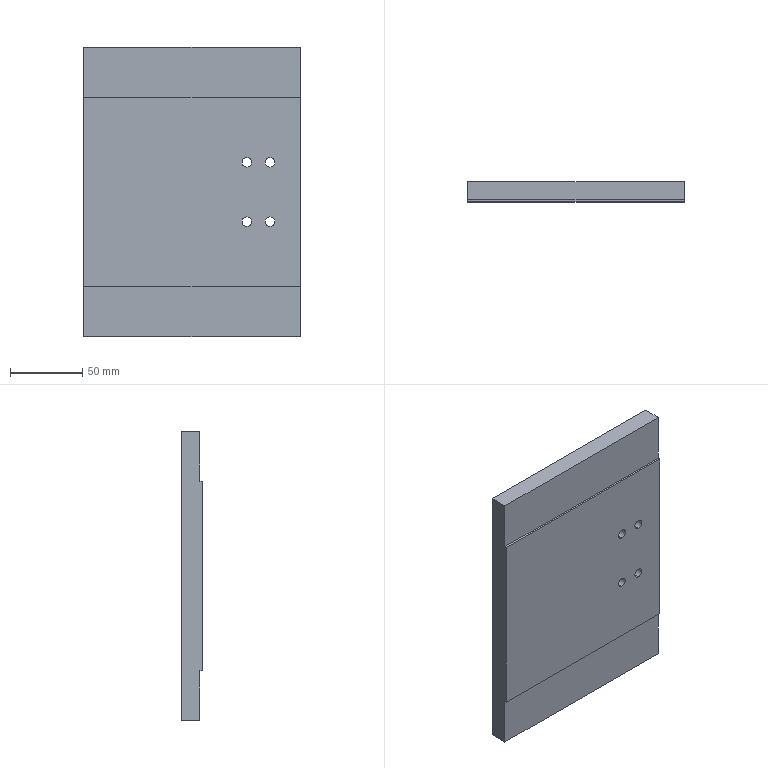Part | SolidWorks | features ICE 2, 3DProfileFeature 1, Extrusion 1, HoleWzd 1 | 1 solid | 30 faces | box 150 x 14 x 200 mm | volume 400905 mm3 | cylinder 16 | plane 14 | commonest cylinder face diameters 6.6 x8 11 x8
STEP:
#1=CARTESIAN_POINT('',(37.95,7.2,15.));
#2=VERTEX_POINT('',#1);
#3=CARTESIAN_POINT('',(37.95,7.2,26.));
#4=VERTEX_POINT('',#3);
#5=CARTESIAN_POINT('',(37.95,7.2,20.5));
#6=DIRECTION('',(0.,1.,0.));
#7=DIRECTION('',(0.,0.,1.));
#8=AXIS2_PLACEMENT_3D('',#5,#6,#7);
#9=CIRCLE('',#8,5.5);
#10=EDGE_CURVE('',#2,#4,#9,.T.);
#11=ORIENTED_EDGE('',*,*,#10,.F.);
#12=CARTESIAN_POINT('',(37.95,14.,15.));
#13=VERTEX_POINT('',#12);
#14=CARTESIAN_POINT('',(37.95,14.,15.));
#15=DIRECTION('',(0.,1.,0.));
#16=VECTOR('',#15,1000.);
#17=LINE('',#14,#16);
#18=EDGE_CURVE('',#2,#13,#17,.T.);
#19=ORIENTED_EDGE('',*,*,#18,.T.);
#20=CARTESIAN_POINT('',(37.95,14.,26.));
#21=VERTEX_POINT('',#20);
#22=CARTESIAN_POINT('',(37.95,14.,20.5));
#23=DIRECTION('',(0.,1.,0.));
#24=DIRECTION('',(0.,0.,1.));
#25=AXIS2_PLACEMENT_3D('',#22,#23,#24);
#26=CIRCLE('',#25,5.5);
#27=EDGE_CURVE('',#13,#21,#26,.T.);
#28=ORIENTED_EDGE('',*,*,#27,.T.);
#29=CARTESIAN_POINT('',(37.95,14.,26.));
#30=DIRECTION('',(0.,1.,0.));
#31=VECTOR('',#30,1000.);
#32=LINE('',#29,#31);
#33=EDGE_CURVE('',#4,#21,#32,.T.);
#34=ORIENTED_EDGE('',*,*,#33,.F.);
#35=EDGE_LOOP('',(#11,#19,#28,#34));
#36=FACE_OUTER_BOUND('',#35,.T.);
#37=CARTESIAN_POINT('',(37.95,14.,20.5));
#38=DIRECTION('',(0.,1.,0.));
#39=DIRECTION('',(0.,0.,1.));
#40=AXIS2_PLACEMENT_3D('',#37,#38,#39);
#41=CYLINDRICAL_SURFACE('',#40,5.5);
#42=ADVANCED_FACE('',(#36),#41,.F.);
#43=CARTESIAN_POINT('',(37.95,0.,23.8));
#44=VERTEX_POINT('',#43);
#45=CARTESIAN_POINT('',(37.95,0.,17.2));
#46=VERTEX_POINT('',#45);
#47=CARTESIAN_POINT('',(37.95,0.,20.5));
#48=DIRECTION('',(0.,-1.,0.));
#49=DIRECTION('',(0.,0.,-1.));
#50=AXIS2_PLACEMENT_3D('',#47,#48,#49);
#51=CIRCLE('',#50,3.3);
#52=EDGE_CURVE('',#44,#46,#51,.T.);
#53=ORIENTED_EDGE('',*,*,#52,.T.);
#54=CARTESIAN_POINT('',(37.95,7.2,17.2));
#55=VERTEX_POINT('',#54);
#56=CARTESIAN_POINT('',(37.95,14.,17.2));
#57=DIRECTION('',(0.,1.,0.));
#58=VECTOR('',#57,1000.);
#59=LINE('',#56,#58);
#60=EDGE_CURVE('',#46,#55,#59,.T.);
#61=ORIENTED_EDGE('',*,*,#60,.T.);
#62=CARTESIAN_POINT('',(37.95,7.2,23.8));
#63=VERTEX_POINT('',#62);
#64=CARTESIAN_POINT('',(37.95,7.2,20.5));
#65=DIRECTION('',(0.,1.,0.));
#66=DIRECTION('',(0.,0.,1.));
#67=AXIS2_PLACEMENT_3D('',#64,#65,#66);
#68=CIRCLE('',#67,3.3);
#69=EDGE_CURVE('',#55,#63,#68,.T.);
#70=ORIENTED_EDGE('',*,*,#69,.T.);
#71=CARTESIAN_POINT('',(37.95,14.,23.8));
#72=DIRECTION('',(0.,1.,0.));
#73=VECTOR('',#72,1000.);
#74=LINE('',#71,#73);
#75=EDGE_CURVE('',#44,#63,#74,.T.);
#76=ORIENTED_EDGE('',*,*,#75,.F.);
#77=EDGE_LOOP('',(#53,#61,#70,#76));
#78=FACE_OUTER_BOUND('',#77,.T.);
#79=CARTESIAN_POINT('',(37.95,14.,20.5));
#80=DIRECTION('',(0.,1.,0.));
#81=DIRECTION('',(0.,0.,1.));
#82=AXIS2_PLACEMENT_3D('',#79,#80,#81);
#83=CYLINDRICAL_SURFACE('',#82,3.3);
#84=ADVANCED_FACE('',(#78),#83,.F.);
#85=CARTESIAN_POINT('',(37.95,7.2,-26.));
#86=VERTEX_POINT('',#85);
#87=CARTESIAN_POINT('',(37.95,7.2,-15.));
#88=VERTEX_POINT('',#87);
#89=CARTESIAN_POINT('',(37.95,7.2,-20.5));
#90=DIRECTION('',(0.,1.,0.));
#91=DIRECTION('',(0.,0.,1.));
#92=AXIS2_PLACEMENT_3D('',#89,#90,#91);
#93=CIRCLE('',#92,5.5);
#94=EDGE_CURVE('',#86,#88,#93,.T.);
#95=ORIENTED_EDGE('',*,*,#94,.F.);
#96=CARTESIAN_POINT('',(37.95,14.,-26.));
#97=VERTEX_POINT('',#96);
#98=CARTESIAN_POINT('',(37.95,14.,-26.));
#99=DIRECTION('',(0.,1.,0.));
#100=VECTOR('',#99,1000.);
#101=LINE('',#98,#100);
#102=EDGE_CURVE('',#86,#97,#101,.T.);
#103=ORIENTED_EDGE('',*,*,#102,.T.);
#104=CARTESIAN_POINT('',(37.95,14.,-15.));
#105=VERTEX_POINT('',#104);
#106=CARTESIAN_POINT('',(37.95,14.,-20.5));
#107=DIRECTION('',(0.,1.,0.));
#108=DIRECTION('',(0.,0.,1.));
#109=AXIS2_PLACEMENT_3D('',#106,#107,#108);
#110=CIRCLE('',#109,5.5);
#111=EDGE_CURVE('',#97,#105,#110,.T.);
#112=ORIENTED_EDGE('',*,*,#111,.T.);
#113=CARTESIAN_POINT('',(37.95,14.,-15.));
#114=DIRECTION('',(0.,1.,0.));
#115=VECTOR('',#114,1000.);
#116=LINE('',#113,#115);
#117=EDGE_CURVE('',#88,#105,#116,.T.);
#118=ORIENTED_EDGE('',*,*,#117,.F.);
#119=EDGE_LOOP('',(#95,#103,#112,#118));
#120=FACE_OUTER_BOUND('',#119,.T.);
#121=CARTESIAN_POINT('',(37.95,14.,-20.5));
#122=DIRECTION('',(0.,1.,0.));
#123=DIRECTION('',(0.,0.,1.));
#124=AXIS2_PLACEMENT_3D('',#121,#122,#123);
#125=CYLINDRICAL_SURFACE('',#124,5.5);
#126=ADVANCED_FACE('',(#120),#125,.F.);
#127=CARTESIAN_POINT('',(37.95,0.,-17.2));
#128=VERTEX_POINT('',#127);
#129=CARTESIAN_POINT('',(37.95,0.,-23.8));
#130=VERTEX_POINT('',#129);
#131=CARTESIAN_POINT('',(37.95,0.,-20.5));
#132=DIRECTION('',(0.,-1.,0.));
#133=DIRECTION('',(0.,0.,-1.));
#134=AXIS2_PLACEMENT_3D('',#131,#132,#133);
#135=CIRCLE('',#134,3.3);
#136=EDGE_CURVE('',#128,#130,#135,.T.);
#137=ORIENTED_EDGE('',*,*,#136,.T.);
#138=CARTESIAN_POINT('',(37.95,7.2,-23.8));
#139=VERTEX_POINT('',#138);
#140=CARTESIAN_POINT('',(37.95,14.,-23.8));
#141=DIRECTION('',(0.,1.,0.));
#142=VECTOR('',#141,1000.);
#143=LINE('',#140,#142);
#144=EDGE_CURVE('',#130,#139,#143,.T.);
#145=ORIENTED_EDGE('',*,*,#144,.T.);
#146=CARTESIAN_POINT('',(37.95,7.2,-17.2));
#147=VERTEX_POINT('',#146);
#148=CARTESIAN_POINT('',(37.95,7.2,-20.5));
#149=DIRECTION('',(0.,1.,0.));
#150=DIRECTION('',(0.,0.,1.));
#151=AXIS2_PLACEMENT_3D('',#148,#149,#150);
#152=CIRCLE('',#151,3.3);
#153=EDGE_CURVE('',#139,#147,#152,.T.);
#154=ORIENTED_EDGE('',*,*,#153,.T.);
#155=CARTESIAN_POINT('',(37.95,14.,-17.2));
#156=DIRECTION('',(0.,1.,0.));
#157=VECTOR('',#156,1000.);
#158=LINE('',#155,#157);
#159=EDGE_CURVE('',#128,#147,#158,.T.);
#160=ORIENTED_EDGE('',*,*,#159,.F.);
#161=EDGE_LOOP('',(#137,#145,#154,#160));
#162=FACE_OUTER_BOUND('',#161,.T.);
#163=CARTESIAN_POINT('',(37.95,14.,-20.5));
#164=DIRECTION('',(0.,1.,0.));
#165=DIRECTION('',(0.,0.,1.));
#166=AXIS2_PLACEMENT_3D('',#163,#164,#165);
#167=CYLINDRICAL_SURFACE('',#166,3.3);
#168=ADVANCED_FACE('',(#162),#167,.F.);
#169=CARTESIAN_POINT('',(53.95,7.2,15.));
#170=VERTEX_POINT('',#169);
#171=CARTESIAN_POINT('',(53.95,7.2,26.));
#172=VERTEX_POINT('',#171);
#173=CARTESIAN_POINT('',(53.95,7.2,20.5));
#174=DIRECTION('',(0.,1.,0.));
#175=DIRECTION('',(0.,0.,1.));
#176=AXIS2_PLACEMENT_3D('',#173,#174,#175);
#177=CIRCLE('',#176,5.5);
#178=EDGE_CURVE('',#170,#172,#177,.T.);
#179=ORIENTED_EDGE('',*,*,#178,.F.);
#180=CARTESIAN_POINT('',(53.95,14.,15.));
#181=VERTEX_POINT('',#180);
#182=CARTESIAN_POINT('',(53.95,14.,15.));
#183=DIRECTION('',(0.,1.,0.));
#184=VECTOR('',#183,1000.);
#185=LINE('',#182,#184);
#186=EDGE_CURVE('',#170,#181,#185,.T.);
#187=ORIENTED_EDGE('',*,*,#186,.T.);
#188=CARTESIAN_POINT('',(53.95,14.,26.));
#189=VERTEX_POINT('',#188);
#190=CARTESIAN_POINT('',(53.95,14.,20.5));
#191=DIRECTION('',(0.,1.,0.));
#192=DIRECTION('',(0.,0.,1.));
#193=AXIS2_PLACEMENT_3D('',#190,#191,#192);
#194=CIRCLE('',#193,5.5);
#195=EDGE_CURVE('',#181,#189,#194,.T.);
#196=ORIENTED_EDGE('',*,*,#195,.T.);
#197=CARTESIAN_POINT('',(53.95,14.,26.));
#198=DIRECTION('',(0.,1.,0.));
#199=VECTOR('',#198,1000.);
#200=LINE('',#197,#199);
#201=EDGE_CURVE('',#172,#189,#200,.T.);
#202=ORIENTED_EDGE('',*,*,#201,.F.);
#203=EDGE_LOOP('',(#179,#187,#196,#202));
#204=FACE_OUTER_BOUND('',#203,.T.);
#205=CARTESIAN_POINT('',(53.95,14.,20.5));
#206=DIRECTION('',(0.,1.,0.));
#207=DIRECTION('',(0.,0.,1.));
#208=AXIS2_PLACEMENT_3D('',#205,#206,#207);
#209=CYLINDRICAL_SURFACE('',#208,5.5);
#210=ADVANCED_FACE('',(#204),#209,.F.);
#211=CARTESIAN_POINT('',(53.95,0.,23.8));
#212=VERTEX_POINT('',#211);
#213=CARTESIAN_POINT('',(53.95,0.,17.2));
#214=VERTEX_POINT('',#213);
#215=CARTESIAN_POINT('',(53.95,0.,20.5));
#216=DIRECTION('',(0.,-1.,0.));
#217=DIRECTION('',(0.,0.,-1.));
#218=AXIS2_PLACEMENT_3D('',#215,#216,#217);
#219=CIRCLE('',#218,3.3);
#220=EDGE_CURVE('',#212,#214,#219,.T.);
#221=ORIENTED_EDGE('',*,*,#220,.T.);
#222=CARTESIAN_POINT('',(53.95,7.2,17.2));
#223=VERTEX_POINT('',#222);
#224=CARTESIAN_POINT('',(53.95,14.,17.2));
#225=DIRECTION('',(0.,1.,0.));
#226=VECTOR('',#225,1000.);
#227=LINE('',#224,#226);
#228=EDGE_CURVE('',#214,#223,#227,.T.);
#229=ORIENTED_EDGE('',*,*,#228,.T.);
#230=CARTESIAN_POINT('',(53.95,7.2,23.8));
#231=VERTEX_POINT('',#230);
#232=CARTESIAN_POINT('',(53.95,7.2,20.5));
#233=DIRECTION('',(0.,1.,0.));
#234=DIRECTION('',(0.,0.,1.));
#235=AXIS2_PLACEMENT_3D('',#232,#233,#234);
#236=CIRCLE('',#235,3.3);
#237=EDGE_CURVE('',#223,#231,#236,.T.);
#238=ORIENTED_EDGE('',*,*,#237,.T.);
#239=CARTESIAN_POINT('',(53.95,14.,23.8));
#240=DIRECTION('',(0.,1.,0.));
#241=VECTOR('',#240,1000.);
#242=LINE('',#239,#241);
#243=EDGE_CURVE('',#212,#231,#242,.T.);
#244=ORIENTED_EDGE('',*,*,#243,.F.);
#245=EDGE_LOOP('',(#221,#229,#238,#244));
#246=FACE_OUTER_BOUND('',#245,.T.);
#247=CARTESIAN_POINT('',(53.95,14.,20.5));
#248=DIRECTION('',(0.,1.,0.));
#249=DIRECTION('',(0.,0.,1.));
#250=AXIS2_PLACEMENT_3D('',#247,#248,#249);
#251=CYLINDRICAL_SURFACE('',#250,3.3);
#252=ADVANCED_FACE('',(#246),#251,.F.);
#253=CARTESIAN_POINT('',(53.95,7.2,-26.));
#254=VERTEX_POINT('',#253);
#255=CARTESIAN_POINT('',(53.95,7.2,-15.));
#256=VERTEX_POINT('',#255);
#257=CARTESIAN_POINT('',(53.95,7.2,-20.5));
#258=DIRECTION('',(0.,1.,0.));
#259=DIRECTION('',(0.,0.,1.));
#260=AXIS2_PLACEMENT_3D('',#257,#258,#259);
#261=CIRCLE('',#260,5.5);
#262=EDGE_CURVE('',#254,#256,#261,.T.);
#263=ORIENTED_EDGE('',*,*,#262,.F.);
#264=CARTESIAN_POINT('',(53.95,14.,-26.));
#265=VERTEX_POINT('',#264);
#266=CARTESIAN_POINT('',(53.95,14.,-26.));
#267=DIRECTION('',(0.,1.,0.));
#268=VECTOR('',#267,1000.);
#269=LINE('',#266,#268);
#270=EDGE_CURVE('',#254,#265,#269,.T.);
#271=ORIENTED_EDGE('',*,*,#270,.T.);
#272=CARTESIAN_POINT('',(53.95,14.,-15.));
#273=VERTEX_POINT('',#272);
#274=CARTESIAN_POINT('',(53.95,14.,-20.5));
#275=DIRECTION('',(0.,1.,0.));
#276=DIRECTION('',(0.,0.,1.));
#277=AXIS2_PLACEMENT_3D('',#274,#275,#276);
#278=CIRCLE('',#277,5.5);
#279=EDGE_CURVE('',#265,#273,#278,.T.);
#280=ORIENTED_EDGE('',*,*,#279,.T.);
#281=CARTESIAN_POINT('',(53.95,14.,-15.));
#282=DIRECTION('',(0.,1.,0.));
#283=VECTOR('',#282,1000.);
#284=LINE('',#281,#283);
#285=EDGE_CURVE('',#256,#273,#284,.T.);
#286=ORIENTED_EDGE('',*,*,#285,.F.);
#287=EDGE_LOOP('',(#263,#271,#280,#286));
#288=FACE_OUTER_BOUND('',#287,.T.);
#289=CARTESIAN_POINT('',(53.95,14.,-20.5));
#290=DIRECTION('',(0.,1.,0.));
#291=DIRECTION('',(0.,0.,1.));
#292=AXIS2_PLACEMENT_3D('',#289,#290,#291);
#293=CYLINDRICAL_SURFACE('',#292,5.5);
#294=ADVANCED_FACE('',(#288),#293,.F.);
#295=CARTESIAN_POINT('',(53.95,0.,-17.2));
#296=VERTEX_POINT('',#295);
#297=CARTESIAN_POINT('',(53.95,0.,-23.8));
#298=VERTEX_POINT('',#297);
#299=CARTESIAN_POINT('',(53.95,0.,-20.5));
#300=DIRECTION('',(0.,-1.,0.));
#301=DIRECTION('',(0.,0.,-1.));
#302=AXIS2_PLACEMENT_3D('',#299,#300,#301);
#303=CIRCLE('',#302,3.3);
#304=EDGE_CURVE('',#296,#298,#303,.T.);
#305=ORIENTED_EDGE('',*,*,#304,.T.);
#306=CARTESIAN_POINT('',(53.95,7.2,-23.8));
#307=VERTEX_POINT('',#306);
#308=CARTESIAN_POINT('',(53.95,14.,-23.8));
#309=DIRECTION('',(0.,1.,0.));
#310=VECTOR('',#309,1000.);
#311=LINE('',#308,#310);
#312=EDGE_CURVE('',#298,#307,#311,.T.);
#313=ORIENTED_EDGE('',*,*,#312,.T.);
#314=CARTESIAN_POINT('',(53.95,7.2,-17.2));
#315=VERTEX_POINT('',#314);
#316=CARTESIAN_POINT('',(53.95,7.2,-20.5));
#317=DIRECTION('',(0.,1.,0.));
#318=DIRECTION('',(0.,0.,1.));
#319=AXIS2_PLACEMENT_3D('',#316,#317,#318);
#320=CIRCLE('',#319,3.3);
#321=EDGE_CURVE('',#307,#315,#320,.T.);
#322=ORIENTED_EDGE('',*,*,#321,.T.);
#323=CARTESIAN_POINT('',(53.95,14.,-17.2));
#324=DIRECTION('',(0.,1.,0.));
#325=VECTOR('',#324,1000.);
#326=LINE('',#323,#325);
#327=EDGE_CURVE('',#296,#315,#326,.T.);
#328=ORIENTED_EDGE('',*,*,#327,.F.);
#329=EDGE_LOOP('',(#305,#313,#322,#328));
#330=FACE_OUTER_BOUND('',#329,.T.);
#331=CARTESIAN_POINT('',(53.95,14.,-20.5));
#332=DIRECTION('',(0.,1.,0.));
#333=DIRECTION('',(0.,0.,1.));
#334=AXIS2_PLACEMENT_3D('',#331,#332,#333);
#335=CYLINDRICAL_SURFACE('',#334,3.3);
#336=ADVANCED_FACE('',(#330),#335,.F.);
#337=CARTESIAN_POINT('',(75.,1.5,100.));
#338=VERTEX_POINT('',#337);
#339=CARTESIAN_POINT('',(-75.,1.5,100.));
#340=VERTEX_POINT('',#339);
#341=CARTESIAN_POINT('',(-75.,1.5,100.));
#342=DIRECTION('',(-1.,0.,0.));
#343=VECTOR('',#342,1000.);
#344=LINE('',#341,#343);
#345=EDGE_CURVE('',#338,#340,#344,.T.);
#346=ORIENTED_EDGE('',*,*,#345,.F.);
#347=CARTESIAN_POINT('',(75.,14.,100.));
#348=VERTEX_POINT('',#347);
#349=CARTESIAN_POINT('',(75.,14.,100.));
#350=DIRECTION('',(0.,-1.,0.));
#351=VECTOR('',#350,1000.);
#352=LINE('',#349,#351);
#353=EDGE_CURVE('',#348,#338,#352,.T.);
#354=ORIENTED_EDGE('',*,*,#353,.F.);
#355=CARTESIAN_POINT('',(-75.,14.,100.));
#356=VERTEX_POINT('',#355);
#357=CARTESIAN_POINT('',(-75.,14.,100.));
#358=DIRECTION('',(1.,0.,0.));
#359=VECTOR('',#358,1000.);
#360=LINE('',#357,#359);
#361=EDGE_CURVE('',#356,#348,#360,.T.);
#362=ORIENTED_EDGE('',*,*,#361,.F.);
#363=CARTESIAN_POINT('',(-75.,14.,100.));
#364=DIRECTION('',(0.,-1.,0.));
#365=VECTOR('',#364,1000.);
#366=LINE('',#363,#365);
#367=EDGE_CURVE('',#356,#340,#366,.T.);
#368=ORIENTED_EDGE('',*,*,#367,.T.);
#369=EDGE_LOOP('',(#346,#354,#362,#368));
#370=FACE_OUTER_BOUND('',#369,.T.);
#371=CARTESIAN_POINT('',(-75.,14.,100.));
#372=DIRECTION('',(0.,0.,-1.));
#373=DIRECTION('',(-1.,0.,0.));
#374=AXIS2_PLACEMENT_3D('',#371,#372,#373);
#375=PLANE('',#374);
#376=ADVANCED_FACE('',(#370),#375,.F.);
#377=CARTESIAN_POINT('',(75.,1.5,65.5));
#378=VERTEX_POINT('',#377);
#379=CARTESIAN_POINT('',(75.,1.5,100.));
#380=DIRECTION('',(0.,0.,1.));
#381=VECTOR('',#380,1000.);
#382=LINE('',#379,#381);
#383=EDGE_CURVE('',#378,#338,#382,.T.);
#384=ORIENTED_EDGE('',*,*,#383,.F.);
#385=CARTESIAN_POINT('',(75.,0.,65.5));
#386=VERTEX_POINT('',#385);
#387=CARTESIAN_POINT('',(75.,1.5,65.5));
#388=DIRECTION('',(0.,-1.,0.));
#389=VECTOR('',#388,1000.);
#390=LINE('',#387,#389);
#391=EDGE_CURVE('',#378,#386,#390,.T.);
#392=ORIENTED_EDGE('',*,*,#391,.T.);
#393=CARTESIAN_POINT('',(75.,0.,-65.5));
#394=VERTEX_POINT('',#393);
#395=CARTESIAN_POINT('',(75.,0.,100.));
#396=DIRECTION('',(0.,0.,-1.));
#397=VECTOR('',#396,1000.);
#398=LINE('',#395,#397);
#399=EDGE_CURVE('',#386,#394,#398,.T.);
#400=ORIENTED_EDGE('',*,*,#399,.T.);
#401=CARTESIAN_POINT('',(75.,1.5,-65.5));
#402=VERTEX_POINT('',#401);
#403=CARTESIAN_POINT('',(75.,1.5,-65.5));
#404=DIRECTION('',(0.,-1.,0.));
#405=VECTOR('',#404,1000.);
#406=LINE('',#403,#405);
#407=EDGE_CURVE('',#402,#394,#406,.T.);
#408=ORIENTED_EDGE('',*,*,#407,.F.);
#409=CARTESIAN_POINT('',(75.,1.5,-100.));
#410=VERTEX_POINT('',#409);
#411=CARTESIAN_POINT('',(75.,1.5,-100.));
#412=DIRECTION('',(0.,0.,1.));
#413=VECTOR('',#412,1000.);
#414=LINE('',#411,#413);
#415=EDGE_CURVE('',#410,#402,#414,.T.);
#416=ORIENTED_EDGE('',*,*,#415,.F.);
#417=CARTESIAN_POINT('',(75.,14.,-100.));
#418=VERTEX_POINT('',#417);
#419=CARTESIAN_POINT('',(75.,14.,-100.));
#420=DIRECTION('',(0.,-1.,0.));
#421=VECTOR('',#420,1000.);
#422=LINE('',#419,#421);
#423=EDGE_CURVE('',#418,#410,#422,.T.);
#424=ORIENTED_EDGE('',*,*,#423,.F.);
#425=CARTESIAN_POINT('',(75.,14.,100.));
#426=DIRECTION('',(0.,0.,-1.));
#427=VECTOR('',#426,1000.);
#428=LINE('',#425,#427);
#429=EDGE_CURVE('',#348,#418,#428,.T.);
#430=ORIENTED_EDGE('',*,*,#429,.F.);
#431=ORIENTED_EDGE('',*,*,#353,.T.);
#432=EDGE_LOOP('',(#384,#392,#400,#408,#416,#424,#430,#431));
#433=FACE_OUTER_BOUND('',#432,.T.);
#434=CARTESIAN_POINT('',(75.,14.,100.));
#435=DIRECTION('',(-1.,0.,0.));
#436=DIRECTION('',(0.,0.,1.));
#437=AXIS2_PLACEMENT_3D('',#434,#435,#436);
#438=PLANE('',#437);
#439=ADVANCED_FACE('',(#433),#438,.F.);
#440=ORIENTED_EDGE('',*,*,#423,.T.);
#441=CARTESIAN_POINT('',(-75.,1.5,-100.));
#442=VERTEX_POINT('',#441);
#443=CARTESIAN_POINT('',(-75.,1.5,-100.));
#444=DIRECTION('',(1.,0.,0.));
#445=VECTOR('',#444,1000.);
#446=LINE('',#443,#445);
#447=EDGE_CURVE('',#442,#410,#446,.T.);
#448=ORIENTED_EDGE('',*,*,#447,.F.);
#449=CARTESIAN_POINT('',(-75.,14.,-100.));
#450=VERTEX_POINT('',#449);
#451=CARTESIAN_POINT('',(-75.,14.,-100.));
#452=DIRECTION('',(0.,-1.,0.));
#453=VECTOR('',#452,1000.);
#454=LINE('',#451,#453);
#455=EDGE_CURVE('',#450,#442,#454,.T.);
#456=ORIENTED_EDGE('',*,*,#455,.F.);
#457=CARTESIAN_POINT('',(-75.,14.,-100.));
#458=DIRECTION('',(-1.,0.,0.));
#459=VECTOR('',#458,1000.);
#460=LINE('',#457,#459);
#461=EDGE_CURVE('',#418,#450,#460,.T.);
#462=ORIENTED_EDGE('',*,*,#461,.F.);
#463=EDGE_LOOP('',(#440,#448,#456,#462));
#464=FACE_OUTER_BOUND('',#463,.T.);
#465=CARTESIAN_POINT('',(-75.,14.,-100.));
#466=DIRECTION('',(0.,0.,1.));
#467=DIRECTION('',(1.,0.,0.));
#468=AXIS2_PLACEMENT_3D('',#465,#466,#467);
#469=PLANE('',#468);
#470=ADVANCED_FACE('',(#464),#469,.F.);
#471=CARTESIAN_POINT('',(-75.,0.,-65.5));
#472=VERTEX_POINT('',#471);
#473=CARTESIAN_POINT('',(-75.,0.,65.5));
#474=VERTEX_POINT('',#473);
#475=CARTESIAN_POINT('',(-75.,0.,100.));
#476=DIRECTION('',(0.,0.,1.));
#477=VECTOR('',#476,1000.);
#478=LINE('',#475,#477);
#479=EDGE_CURVE('',#472,#474,#478,.T.);
#480=ORIENTED_EDGE('',*,*,#479,.T.);
#481=CARTESIAN_POINT('',(-75.,1.5,65.5));
#482=VERTEX_POINT('',#481);
#483=CARTESIAN_POINT('',(-75.,1.5,65.5));
#484=DIRECTION('',(0.,-1.,0.));
#485=VECTOR('',#484,1000.);
#486=LINE('',#483,#485);
#487=EDGE_CURVE('',#482,#474,#486,.T.);
#488=ORIENTED_EDGE('',*,*,#487,.F.);
#489=CARTESIAN_POINT('',(-75.,1.5,100.));
#490=DIRECTION('',(0.,0.,-1.));
#491=VECTOR('',#490,1000.);
#492=LINE('',#489,#491);
#493=EDGE_CURVE('',#340,#482,#492,.T.);
#494=ORIENTED_EDGE('',*,*,#493,.F.);
#495=ORIENTED_EDGE('',*,*,#367,.F.);
#496=CARTESIAN_POINT('',(-75.,14.,100.));
#497=DIRECTION('',(0.,0.,1.));
#498=VECTOR('',#497,1000.);
#499=LINE('',#496,#498);
#500=EDGE_CURVE('',#450,#356,#499,.T.);
#501=ORIENTED_EDGE('',*,*,#500,.F.);
#502=ORIENTED_EDGE('',*,*,#455,.T.);
#503=CARTESIAN_POINT('',(-75.,1.5,-65.5));
#504=VERTEX_POINT('',#503);
#505=CARTESIAN_POINT('',(-75.,1.5,-100.));
#506=DIRECTION('',(0.,0.,-1.));
#507=VECTOR('',#506,1000.);
#508=LINE('',#505,#507);
#509=EDGE_CURVE('',#504,#442,#508,.T.);
#510=ORIENTED_EDGE('',*,*,#509,.F.);
#511=CARTESIAN_POINT('',(-75.,1.5,-65.5));
#512=DIRECTION('',(0.,-1.,0.));
#513=VECTOR('',#512,1000.);
#514=LINE('',#511,#513);
#515=EDGE_CURVE('',#504,#472,#514,.T.);
#516=ORIENTED_EDGE('',*,*,#515,.T.);
#517=EDGE_LOOP('',(#480,#488,#494,#495,#501,#502,#510,#516));
#518=FACE_OUTER_BOUND('',#517,.T.);
#519=CARTESIAN_POINT('',(-75.,14.,100.));
#520=DIRECTION('',(1.,0.,0.));
#521=DIRECTION('',(0.,0.,-1.));
#522=AXIS2_PLACEMENT_3D('',#519,#520,#521);
#523=PLANE('',#522);
#524=ADVANCED_FACE('',(#518),#523,.F.);
#525=CARTESIAN_POINT('',(37.95,14.,20.5));
#526=DIRECTION('',(0.,1.,0.));
#527=DIRECTION('',(0.,0.,1.));
#528=AXIS2_PLACEMENT_3D('',#525,#526,#527);
#529=CIRCLE('',#528,5.5);
#530=EDGE_CURVE('',#21,#13,#529,.T.);
#531=ORIENTED_EDGE('',*,*,#530,.F.);
#532=ORIENTED_EDGE('',*,*,#27,.F.);
#533=EDGE_LOOP('',(#531,#532));
#534=FACE_BOUND('',#533,.T.);
#535=CARTESIAN_POINT('',(37.95,14.,-20.5));
#536=DIRECTION('',(0.,1.,0.));
#537=DIRECTION('',(0.,0.,1.));
#538=AXIS2_PLACEMENT_3D('',#535,#536,#537);
#539=CIRCLE('',#538,5.5);
#540=EDGE_CURVE('',#105,#97,#539,.T.);
#541=ORIENTED_EDGE('',*,*,#540,.F.);
#542=ORIENTED_EDGE('',*,*,#111,.F.);
#543=EDGE_LOOP('',(#541,#542));
#544=FACE_BOUND('',#543,.T.);
#545=CARTESIAN_POINT('',(53.95,14.,20.5));
#546=DIRECTION('',(0.,1.,0.));
#547=DIRECTION('',(0.,0.,1.));
#548=AXIS2_PLACEMENT_3D('',#545,#546,#547);
#549=CIRCLE('',#548,5.5);
#550=EDGE_CURVE('',#189,#181,#549,.T.);
#551=ORIENTED_EDGE('',*,*,#550,.F.);
#552=ORIENTED_EDGE('',*,*,#195,.F.);
#553=EDGE_LOOP('',(#551,#552));
#554=FACE_BOUND('',#553,.T.);
#555=CARTESIAN_POINT('',(53.95,14.,-20.5));
#556=DIRECTION('',(0.,1.,0.));
#557=DIRECTION('',(0.,0.,1.));
#558=AXIS2_PLACEMENT_3D('',#555,#556,#557);
#559=CIRCLE('',#558,5.5);
#560=EDGE_CURVE('',#273,#265,#559,.T.);
#561=ORIENTED_EDGE('',*,*,#560,.F.);
#562=ORIENTED_EDGE('',*,*,#279,.F.);
#563=EDGE_LOOP('',(#561,#562));
#564=FACE_BOUND('',#563,.T.);
#565=ORIENTED_EDGE('',*,*,#429,.T.);
#566=ORIENTED_EDGE('',*,*,#461,.T.);
#567=ORIENTED_EDGE('',*,*,#500,.T.);
#568=ORIENTED_EDGE('',*,*,#361,.T.);
#569=EDGE_LOOP('',(#565,#566,#567,#568));
#570=FACE_OUTER_BOUND('',#569,.T.);
#571=CARTESIAN_POINT('',(0.,14.,0.));
#572=DIRECTION('',(0.,-1.,0.));
#573=DIRECTION('',(0.,0.,-1.));
#574=AXIS2_PLACEMENT_3D('',#571,#572,#573);
#575=PLANE('',#574);
#576=ADVANCED_FACE('',(#534,#544,#554,#564,#570),#575,.F.);
#577=ORIENTED_EDGE('',*,*,#52,.F.);
#578=CARTESIAN_POINT('',(37.95,0.,20.5));
#579=DIRECTION('',(0.,-1.,0.));
#580=DIRECTION('',(0.,0.,-1.));
#581=AXIS2_PLACEMENT_3D('',#578,#579,#580);
#582=CIRCLE('',#581,3.3);
#583=EDGE_CURVE('',#46,#44,#582,.T.);
#584=ORIENTED_EDGE('',*,*,#583,.F.);
#585=EDGE_LOOP('',(#577,#584));
#586=FACE_BOUND('',#585,.T.);
#587=ORIENTED_EDGE('',*,*,#136,.F.);
#588=CARTESIAN_POINT('',(37.95,0.,-20.5));
#589=DIRECTION('',(0.,-1.,0.));
#590=DIRECTION('',(0.,0.,-1.));
#591=AXIS2_PLACEMENT_3D('',#588,#589,#590);
#592=CIRCLE('',#591,3.3);
#593=EDGE_CURVE('',#130,#128,#592,.T.);
#594=ORIENTED_EDGE('',*,*,#593,.F.);
#595=EDGE_LOOP('',(#587,#594));
#596=FACE_BOUND('',#595,.T.);
#597=ORIENTED_EDGE('',*,*,#220,.F.);
#598=CARTESIAN_POINT('',(53.95,0.,20.5));
#599=DIRECTION('',(0.,-1.,0.));
#600=DIRECTION('',(0.,0.,-1.));
#601=AXIS2_PLACEMENT_3D('',#598,#599,#600);
#602=CIRCLE('',#601,3.3);
#603=EDGE_CURVE('',#214,#212,#602,.T.);
#604=ORIENTED_EDGE('',*,*,#603,.F.);
#605=EDGE_LOOP('',(#597,#604));
#606=FACE_BOUND('',#605,.T.);
#607=ORIENTED_EDGE('',*,*,#304,.F.);
#608=CARTESIAN_POINT('',(53.95,0.,-20.5));
#609=DIRECTION('',(0.,-1.,0.));
#610=DIRECTION('',(0.,0.,-1.));
#611=AXIS2_PLACEMENT_3D('',#608,#609,#610);
#612=CIRCLE('',#611,3.3);
#613=EDGE_CURVE('',#298,#296,#612,.T.);
#614=ORIENTED_EDGE('',*,*,#613,.F.);
#615=EDGE_LOOP('',(#607,#614));
#616=FACE_BOUND('',#615,.T.);
#617=CARTESIAN_POINT('',(-75.,0.,65.5));
#618=DIRECTION('',(1.,0.,0.));
#619=VECTOR('',#618,1000.);
#620=LINE('',#617,#619);
#621=EDGE_CURVE('',#474,#386,#620,.T.);
#622=ORIENTED_EDGE('',*,*,#621,.F.);
#623=ORIENTED_EDGE('',*,*,#479,.F.);
#624=CARTESIAN_POINT('',(-75.,0.,-65.5));
#625=DIRECTION('',(-1.,0.,0.));
#626=VECTOR('',#625,1000.);
#627=LINE('',#624,#626);
#628=EDGE_CURVE('',#394,#472,#627,.T.);
#629=ORIENTED_EDGE('',*,*,#628,.F.);
#630=ORIENTED_EDGE('',*,*,#399,.F.);
#631=EDGE_LOOP('',(#622,#623,#629,#630));
#632=FACE_OUTER_BOUND('',#631,.T.);
#633=CARTESIAN_POINT('',(0.,0.,0.));
#634=DIRECTION('',(0.,-1.,0.));
#635=DIRECTION('',(0.,0.,-1.));
#636=AXIS2_PLACEMENT_3D('',#633,#634,#635);
#637=PLANE('',#636);
#638=ADVANCED_FACE('',(#586,#596,#606,#616,#632),#637,.T.);
#639=ORIENTED_EDGE('',*,*,#628,.T.);
#640=ORIENTED_EDGE('',*,*,#515,.F.);
#641=CARTESIAN_POINT('',(-75.,1.5,-65.5));
#642=DIRECTION('',(-1.,0.,0.));
#643=VECTOR('',#642,1000.);
#644=LINE('',#641,#643);
#645=EDGE_CURVE('',#402,#504,#644,.T.);
#646=ORIENTED_EDGE('',*,*,#645,.F.);
#647=ORIENTED_EDGE('',*,*,#407,.T.);
#648=EDGE_LOOP('',(#639,#640,#646,#647));
#649=FACE_OUTER_BOUND('',#648,.T.);
#650=CARTESIAN_POINT('',(-75.,1.5,-65.5));
#651=DIRECTION('',(0.,0.,1.));
#652=DIRECTION('',(1.,0.,0.));
#653=AXIS2_PLACEMENT_3D('',#650,#651,#652);
#654=PLANE('',#653);
#655=ADVANCED_FACE('',(#649),#654,.F.);
#656=ORIENTED_EDGE('',*,*,#509,.T.);
#657=ORIENTED_EDGE('',*,*,#447,.T.);
#658=ORIENTED_EDGE('',*,*,#415,.T.);
#659=ORIENTED_EDGE('',*,*,#645,.T.);
#660=EDGE_LOOP('',(#656,#657,#658,#659));
#661=FACE_OUTER_BOUND('',#660,.T.);
#662=CARTESIAN_POINT('',(0.,1.5,0.));
#663=DIRECTION('',(0.,1.,0.));
#664=DIRECTION('',(0.,0.,1.));
#665=AXIS2_PLACEMENT_3D('',#662,#663,#664);
#666=PLANE('',#665);
#667=ADVANCED_FACE('',(#661),#666,.F.);
#668=ORIENTED_EDGE('',*,*,#621,.T.);
#669=ORIENTED_EDGE('',*,*,#391,.F.);
#670=CARTESIAN_POINT('',(-75.,1.5,65.5));
#671=DIRECTION('',(1.,0.,0.));
#672=VECTOR('',#671,1000.);
#673=LINE('',#670,#672);
#674=EDGE_CURVE('',#482,#378,#673,.T.);
#675=ORIENTED_EDGE('',*,*,#674,.F.);
#676=ORIENTED_EDGE('',*,*,#487,.T.);
#677=EDGE_LOOP('',(#668,#669,#675,#676));
#678=FACE_OUTER_BOUND('',#677,.T.);
#679=CARTESIAN_POINT('',(-75.,1.5,65.5));
#680=DIRECTION('',(0.,0.,-1.));
#681=DIRECTION('',(-1.,0.,0.));
#682=AXIS2_PLACEMENT_3D('',#679,#680,#681);
#683=PLANE('',#682);
#684=ADVANCED_FACE('',(#678),#683,.F.);
#685=ORIENTED_EDGE('',*,*,#493,.T.);
#686=ORIENTED_EDGE('',*,*,#674,.T.);
#687=ORIENTED_EDGE('',*,*,#383,.T.);
#688=ORIENTED_EDGE('',*,*,#345,.T.);
#689=EDGE_LOOP('',(#685,#686,#687,#688));
#690=FACE_OUTER_BOUND('',#689,.T.);
#691=CARTESIAN_POINT('',(0.,1.5,0.));
#692=DIRECTION('',(0.,-1.,0.));
#693=DIRECTION('',(0.,0.,-1.));
#694=AXIS2_PLACEMENT_3D('',#691,#692,#693);
#695=PLANE('',#694);
#696=ADVANCED_FACE('',(#690),#695,.T.);
#697=ORIENTED_EDGE('',*,*,#312,.F.);
#698=ORIENTED_EDGE('',*,*,#613,.T.);
#699=ORIENTED_EDGE('',*,*,#327,.T.);
#700=CARTESIAN_POINT('',(53.95,7.2,-20.5));
#701=DIRECTION('',(0.,1.,0.));
#702=DIRECTION('',(0.,0.,1.));
#703=AXIS2_PLACEMENT_3D('',#700,#701,#702);
#704=CIRCLE('',#703,3.3);
#705=EDGE_CURVE('',#315,#307,#704,.T.);
#706=ORIENTED_EDGE('',*,*,#705,.T.);
#707=EDGE_LOOP('',(#697,#698,#699,#706));
#708=FACE_OUTER_BOUND('',#707,.T.);
#709=CARTESIAN_POINT('',(53.95,14.,-20.5));
#710=DIRECTION('',(0.,1.,0.));
#711=DIRECTION('',(0.,0.,1.));
#712=AXIS2_PLACEMENT_3D('',#709,#710,#711);
#713=CYLINDRICAL_SURFACE('',#712,3.3);
#714=ADVANCED_FACE('',(#708),#713,.F.);
#715=ORIENTED_EDGE('',*,*,#705,.F.);
#716=ORIENTED_EDGE('',*,*,#321,.F.);
#717=EDGE_LOOP('',(#715,#716));
#718=FACE_BOUND('',#717,.T.);
#719=CARTESIAN_POINT('',(53.95,7.2,-20.5));
#720=DIRECTION('',(0.,1.,0.));
#721=DIRECTION('',(0.,0.,1.));
#722=AXIS2_PLACEMENT_3D('',#719,#720,#721);
#723=CIRCLE('',#722,5.5);
#724=EDGE_CURVE('',#256,#254,#723,.T.);
#725=ORIENTED_EDGE('',*,*,#724,.T.);
#726=ORIENTED_EDGE('',*,*,#262,.T.);
#727=EDGE_LOOP('',(#725,#726));
#728=FACE_OUTER_BOUND('',#727,.T.);
#729=CARTESIAN_POINT('',(57.25,7.2,-20.5));
#730=DIRECTION('',(0.,-1.,0.));
#731=DIRECTION('',(0.,0.,-1.));
#732=AXIS2_PLACEMENT_3D('',#729,#730,#731);
#733=PLANE('',#732);
#734=ADVANCED_FACE('',(#718,#728),#733,.F.);
#735=ORIENTED_EDGE('',*,*,#270,.F.);
#736=ORIENTED_EDGE('',*,*,#724,.F.);
#737=ORIENTED_EDGE('',*,*,#285,.T.);
#738=ORIENTED_EDGE('',*,*,#560,.T.);
#739=EDGE_LOOP('',(#735,#736,#737,#738));
#740=FACE_OUTER_BOUND('',#739,.T.);
#741=CARTESIAN_POINT('',(53.95,14.,-20.5));
#742=DIRECTION('',(0.,1.,0.));
#743=DIRECTION('',(0.,0.,1.));
#744=AXIS2_PLACEMENT_3D('',#741,#742,#743);
#745=CYLINDRICAL_SURFACE('',#744,5.5);
#746=ADVANCED_FACE('',(#740),#745,.F.);
#747=ORIENTED_EDGE('',*,*,#228,.F.);
#748=ORIENTED_EDGE('',*,*,#603,.T.);
#749=ORIENTED_EDGE('',*,*,#243,.T.);
#750=CARTESIAN_POINT('',(53.95,7.2,20.5));
#751=DIRECTION('',(0.,1.,0.));
#752=DIRECTION('',(0.,0.,1.));
#753=AXIS2_PLACEMENT_3D('',#750,#751,#752);
#754=CIRCLE('',#753,3.3);
#755=EDGE_CURVE('',#231,#223,#754,.T.);
#756=ORIENTED_EDGE('',*,*,#755,.T.);
#757=EDGE_LOOP('',(#747,#748,#749,#756));
#758=FACE_OUTER_BOUND('',#757,.T.);
#759=CARTESIAN_POINT('',(53.95,14.,20.5));
#760=DIRECTION('',(0.,1.,0.));
#761=DIRECTION('',(0.,0.,1.));
#762=AXIS2_PLACEMENT_3D('',#759,#760,#761);
#763=CYLINDRICAL_SURFACE('',#762,3.3);
#764=ADVANCED_FACE('',(#758),#763,.F.);
#765=ORIENTED_EDGE('',*,*,#755,.F.);
#766=ORIENTED_EDGE('',*,*,#237,.F.);
#767=EDGE_LOOP('',(#765,#766));
#768=FACE_BOUND('',#767,.T.);
#769=CARTESIAN_POINT('',(53.95,7.2,20.5));
#770=DIRECTION('',(0.,1.,0.));
#771=DIRECTION('',(0.,0.,1.));
#772=AXIS2_PLACEMENT_3D('',#769,#770,#771);
#773=CIRCLE('',#772,5.5);
#774=EDGE_CURVE('',#172,#170,#773,.T.);
#775=ORIENTED_EDGE('',*,*,#774,.T.);
#776=ORIENTED_EDGE('',*,*,#178,.T.);
#777=EDGE_LOOP('',(#775,#776));
#778=FACE_OUTER_BOUND('',#777,.T.);
#779=CARTESIAN_POINT('',(57.25,7.2,20.5));
#780=DIRECTION('',(0.,-1.,0.));
#781=DIRECTION('',(0.,0.,-1.));
#782=AXIS2_PLACEMENT_3D('',#779,#780,#781);
#783=PLANE('',#782);
#784=ADVANCED_FACE('',(#768,#778),#783,.F.);
#785=ORIENTED_EDGE('',*,*,#186,.F.);
#786=ORIENTED_EDGE('',*,*,#774,.F.);
#787=ORIENTED_EDGE('',*,*,#201,.T.);
#788=ORIENTED_EDGE('',*,*,#550,.T.);
#789=EDGE_LOOP('',(#785,#786,#787,#788));
#790=FACE_OUTER_BOUND('',#789,.T.);
#791=CARTESIAN_POINT('',(53.95,14.,20.5));
#792=DIRECTION('',(0.,1.,0.));
#793=DIRECTION('',(0.,0.,1.));
#794=AXIS2_PLACEMENT_3D('',#791,#792,#793);
#795=CYLINDRICAL_SURFACE('',#794,5.5);
#796=ADVANCED_FACE('',(#790),#795,.F.);
#797=ORIENTED_EDGE('',*,*,#144,.F.);
#798=ORIENTED_EDGE('',*,*,#593,.T.);
#799=ORIENTED_EDGE('',*,*,#159,.T.);
#800=CARTESIAN_POINT('',(37.95,7.2,-20.5));
#801=DIRECTION('',(0.,1.,0.));
#802=DIRECTION('',(0.,0.,1.));
#803=AXIS2_PLACEMENT_3D('',#800,#801,#802);
#804=CIRCLE('',#803,3.3);
#805=EDGE_CURVE('',#147,#139,#804,.T.);
#806=ORIENTED_EDGE('',*,*,#805,.T.);
#807=EDGE_LOOP('',(#797,#798,#799,#806));
#808=FACE_OUTER_BOUND('',#807,.T.);
#809=CARTESIAN_POINT('',(37.95,14.,-20.5));
#810=DIRECTION('',(0.,1.,0.));
#811=DIRECTION('',(0.,0.,1.));
#812=AXIS2_PLACEMENT_3D('',#809,#810,#811);
#813=CYLINDRICAL_SURFACE('',#812,3.3);
#814=ADVANCED_FACE('',(#808),#813,.F.);
#815=ORIENTED_EDGE('',*,*,#805,.F.);
#816=ORIENTED_EDGE('',*,*,#153,.F.);
#817=EDGE_LOOP('',(#815,#816));
#818=FACE_BOUND('',#817,.T.);
#819=CARTESIAN_POINT('',(37.95,7.2,-20.5));
#820=DIRECTION('',(0.,1.,0.));
#821=DIRECTION('',(0.,0.,1.));
#822=AXIS2_PLACEMENT_3D('',#819,#820,#821);
#823=CIRCLE('',#822,5.5);
#824=EDGE_CURVE('',#88,#86,#823,.T.);
#825=ORIENTED_EDGE('',*,*,#824,.T.);
#826=ORIENTED_EDGE('',*,*,#94,.T.);
#827=EDGE_LOOP('',(#825,#826));
#828=FACE_OUTER_BOUND('',#827,.T.);
#829=CARTESIAN_POINT('',(41.25,7.2,-20.5));
#830=DIRECTION('',(0.,-1.,0.));
#831=DIRECTION('',(0.,0.,-1.));
#832=AXIS2_PLACEMENT_3D('',#829,#830,#831);
#833=PLANE('',#832);
#834=ADVANCED_FACE('',(#818,#828),#833,.F.);
#835=ORIENTED_EDGE('',*,*,#102,.F.);
#836=ORIENTED_EDGE('',*,*,#824,.F.);
#837=ORIENTED_EDGE('',*,*,#117,.T.);
#838=ORIENTED_EDGE('',*,*,#540,.T.);
#839=EDGE_LOOP('',(#835,#836,#837,#838));
#840=FACE_OUTER_BOUND('',#839,.T.);
#841=CARTESIAN_POINT('',(37.95,14.,-20.5));
#842=DIRECTION('',(0.,1.,0.));
#843=DIRECTION('',(0.,0.,1.));
#844=AXIS2_PLACEMENT_3D('',#841,#842,#843);
#845=CYLINDRICAL_SURFACE('',#844,5.5);
#846=ADVANCED_FACE('',(#840),#845,.F.);
#847=ORIENTED_EDGE('',*,*,#60,.F.);
#848=ORIENTED_EDGE('',*,*,#583,.T.);
#849=ORIENTED_EDGE('',*,*,#75,.T.);
#850=CARTESIAN_POINT('',(37.95,7.2,20.5));
#851=DIRECTION('',(0.,1.,0.));
#852=DIRECTION('',(0.,0.,1.));
#853=AXIS2_PLACEMENT_3D('',#850,#851,#852);
#854=CIRCLE('',#853,3.3);
#855=EDGE_CURVE('',#63,#55,#854,.T.);
#856=ORIENTED_EDGE('',*,*,#855,.T.);
#857=EDGE_LOOP('',(#847,#848,#849,#856));
#858=FACE_OUTER_BOUND('',#857,.T.);
#859=CARTESIAN_POINT('',(37.95,14.,20.5));
#860=DIRECTION('',(0.,1.,0.));
#861=DIRECTION('',(0.,0.,1.));
#862=AXIS2_PLACEMENT_3D('',#859,#860,#861);
#863=CYLINDRICAL_SURFACE('',#862,3.3);
#864=ADVANCED_FACE('',(#858),#863,.F.);
#865=ORIENTED_EDGE('',*,*,#855,.F.);
#866=ORIENTED_EDGE('',*,*,#69,.F.);
#867=EDGE_LOOP('',(#865,#866));
#868=FACE_BOUND('',#867,.T.);
#869=CARTESIAN_POINT('',(37.95,7.2,20.5));
#870=DIRECTION('',(0.,1.,0.));
#871=DIRECTION('',(0.,0.,1.));
#872=AXIS2_PLACEMENT_3D('',#869,#870,#871);
#873=CIRCLE('',#872,5.5);
#874=EDGE_CURVE('',#4,#2,#873,.T.);
#875=ORIENTED_EDGE('',*,*,#874,.T.);
#876=ORIENTED_EDGE('',*,*,#10,.T.);
#877=EDGE_LOOP('',(#875,#876));
#878=FACE_OUTER_BOUND('',#877,.T.);
#879=CARTESIAN_POINT('',(41.25,7.2,20.5));
#880=DIRECTION('',(0.,-1.,0.));
#881=DIRECTION('',(0.,0.,-1.));
#882=AXIS2_PLACEMENT_3D('',#879,#880,#881);
#883=PLANE('',#882);
#884=ADVANCED_FACE('',(#868,#878),#883,.F.);
#885=ORIENTED_EDGE('',*,*,#18,.F.);
#886=ORIENTED_EDGE('',*,*,#874,.F.);
#887=ORIENTED_EDGE('',*,*,#33,.T.);
#888=ORIENTED_EDGE('',*,*,#530,.T.);
#889=EDGE_LOOP('',(#885,#886,#887,#888));
#890=FACE_OUTER_BOUND('',#889,.T.);
#891=CARTESIAN_POINT('',(37.95,14.,20.5));
#892=DIRECTION('',(0.,1.,0.));
#893=DIRECTION('',(0.,0.,1.));
#894=AXIS2_PLACEMENT_3D('',#891,#892,#893);
#895=CYLINDRICAL_SURFACE('',#894,5.5);
#896=ADVANCED_FACE('',(#890),#895,.F.);
#897=CLOSED_SHELL('',(#42,#84,#126,#168,#210,#252,#294,#336,#376,#439,#470,#524,#576,#638,#655,#667,#684,#696,#714,#734,#746,#764,#784,#796,#814,#834,#846,#864,#884,#896));
#898=MANIFOLD_SOLID_BREP('',#897);
#899=CARTESIAN_POINT('',(0.,0.,0.));
#900=DIRECTION('',(0.,0.,1.));
#901=DIRECTION('',(1.,0.,0.));
#902=AXIS2_PLACEMENT_3D('',#899,#900,#901);
#903=(LENGTH_UNIT()NAMED_UNIT(*)SI_UNIT(.MILLI.,.METRE.));
#904=UNCERTAINTY_MEASURE_WITH_UNIT(LENGTH_MEASURE(0.00001),#903,'','');
#905=(NAMED_UNIT(*)PLANE_ANGLE_UNIT()SI_UNIT($,.RADIAN.));
#906=(NAMED_UNIT(*)SI_UNIT($,.STERADIAN.)SOLID_ANGLE_UNIT());
#907=(GEOMETRIC_REPRESENTATION_CONTEXT(3)GLOBAL_UNCERTAINTY_ASSIGNED_CONTEXT((#904))GLOBAL_UNIT_ASSIGNED_CONTEXT((#903,#905,#906))REPRESENTATION_CONTEXT('',''));
#908=ADVANCED_BREP_SHAPE_REPRESENTATION('',(#898,#902),#907);